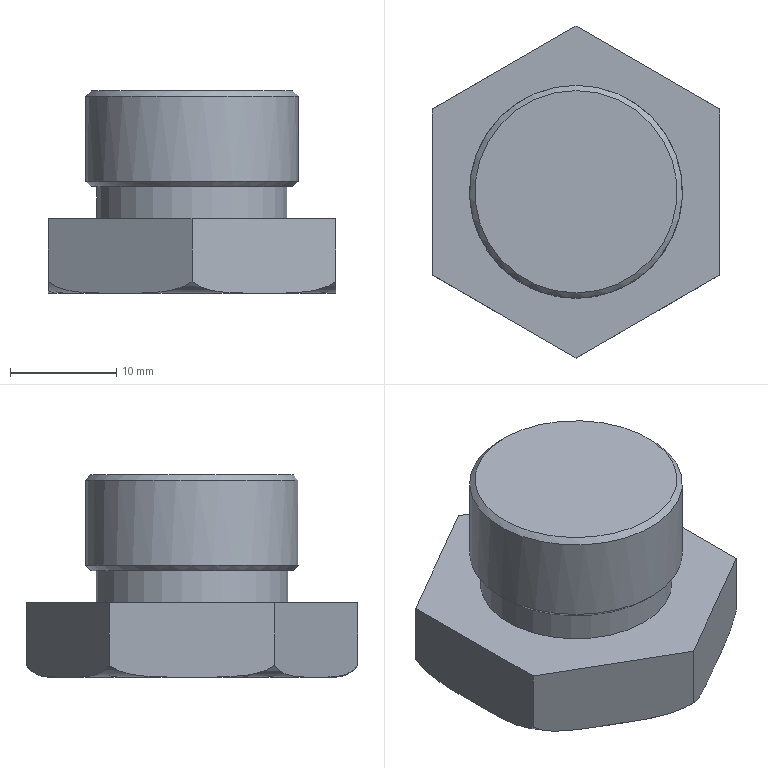Part | STEP file | 3521-20_plug 20 | 1 solid | 20 faces | box 27 x 31.177 x 19.002 mm | volume 7988 mm3 | plane 10 | torus 6 | cylinder 2 | cone 2 | commonest cylinder face diameters 18 x1 20 x1